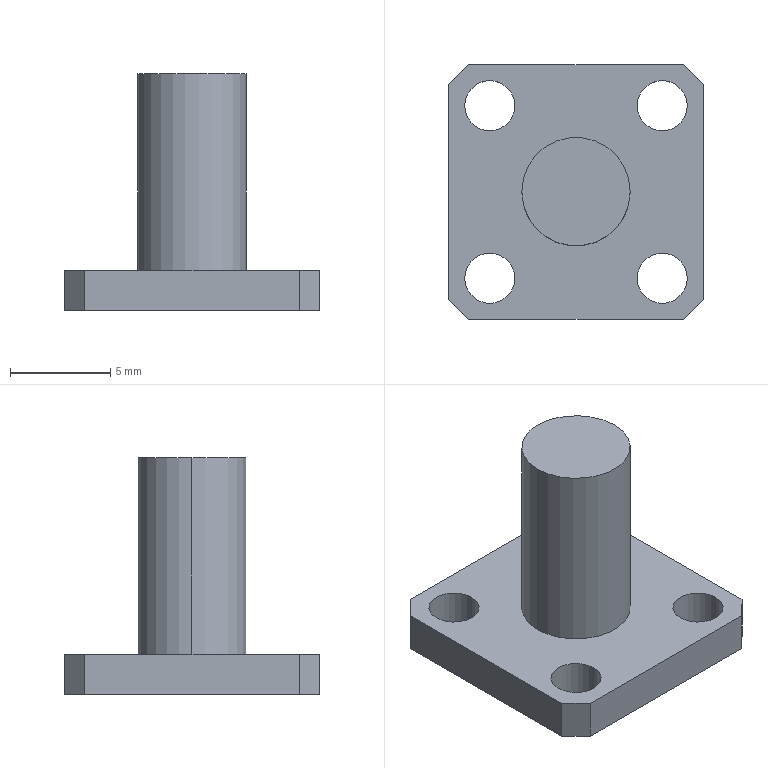Part | SolidWorks | features ICE 2, Chamfer 1, Extrusion 1 | 1 solid | 21 faces | box 12.7 x 12.7 x 11.8 mm | volume 503.752 mm3 | plane 11 | cylinder 10 | commonest cylinder face diameters 2.5 x8 5.4 x2
STEP:
#1=CARTESIAN_POINT('',(-3.65,-6.35,11.8));
#2=VERTEX_POINT('',#1);
#3=CARTESIAN_POINT('',(-9.05,-6.35,11.8));
#4=VERTEX_POINT('',#3);
#5=CARTESIAN_POINT('',(-6.35,-6.35,11.8));
#6=DIRECTION('',(0.,0.,1.));
#7=DIRECTION('',(1.,0.,0.));
#8=AXIS2_PLACEMENT_3D('',#5,#6,#7);
#9=CIRCLE('',#8,2.7);
#10=EDGE_CURVE('',#2,#4,#9,.T.);
#11=ORIENTED_EDGE('',*,*,#10,.F.);
#12=CARTESIAN_POINT('',(-3.65,-6.35,2.));
#13=VERTEX_POINT('',#12);
#14=CARTESIAN_POINT('',(-3.65,-6.35,6.6));
#15=DIRECTION('',(0.,0.,-1.));
#16=VECTOR('',#15,1000.);
#17=LINE('',#14,#16);
#18=EDGE_CURVE('',#2,#13,#17,.T.);
#19=ORIENTED_EDGE('',*,*,#18,.T.);
#20=CARTESIAN_POINT('',(-9.05,-6.35,2.));
#21=VERTEX_POINT('',#20);
#22=CARTESIAN_POINT('',(-6.35,-6.35,2.));
#23=DIRECTION('',(0.,0.,1.));
#24=DIRECTION('',(1.,0.,0.));
#25=AXIS2_PLACEMENT_3D('',#22,#23,#24);
#26=CIRCLE('',#25,2.7);
#27=EDGE_CURVE('',#13,#21,#26,.T.);
#28=ORIENTED_EDGE('',*,*,#27,.T.);
#29=CARTESIAN_POINT('',(-9.05,-6.35,6.6));
#30=DIRECTION('',(0.,0.,-1.));
#31=VECTOR('',#30,1000.);
#32=LINE('',#29,#31);
#33=EDGE_CURVE('',#4,#21,#32,.T.);
#34=ORIENTED_EDGE('',*,*,#33,.F.);
#35=EDGE_LOOP('',(#11,#19,#28,#34));
#36=FACE_OUTER_BOUND('',#35,.T.);
#37=CARTESIAN_POINT('',(-6.35,-6.35,6.6));
#38=DIRECTION('',(0.,0.,-1.));
#39=DIRECTION('',(-1.,0.,0.));
#40=AXIS2_PLACEMENT_3D('',#37,#38,#39);
#41=CYLINDRICAL_SURFACE('',#40,2.7);
#42=ADVANCED_FACE('',(#36),#41,.T.);
#43=CARTESIAN_POINT('',(-11.9,-10.65,2.));
#44=VERTEX_POINT('',#43);
#45=CARTESIAN_POINT('',(-9.4,-10.65,2.));
#46=VERTEX_POINT('',#45);
#47=CARTESIAN_POINT('',(-10.65,-10.65,2.));
#48=DIRECTION('',(0.,0.,1.));
#49=DIRECTION('',(-1.,0.,0.));
#50=AXIS2_PLACEMENT_3D('',#47,#48,#49);
#51=CIRCLE('',#50,1.25);
#52=EDGE_CURVE('',#44,#46,#51,.T.);
#53=ORIENTED_EDGE('',*,*,#52,.T.);
#54=CARTESIAN_POINT('',(-9.4,-10.65,0.));
#55=VERTEX_POINT('',#54);
#56=CARTESIAN_POINT('',(-9.4,-10.65,2.));
#57=DIRECTION('',(0.,0.,-1.));
#58=VECTOR('',#57,1000.);
#59=LINE('',#56,#58);
#60=EDGE_CURVE('',#46,#55,#59,.T.);
#61=ORIENTED_EDGE('',*,*,#60,.T.);
#62=CARTESIAN_POINT('',(-11.9,-10.65,0.));
#63=VERTEX_POINT('',#62);
#64=CARTESIAN_POINT('',(-10.65,-10.65,0.));
#65=DIRECTION('',(0.,0.,1.));
#66=DIRECTION('',(-1.,0.,0.));
#67=AXIS2_PLACEMENT_3D('',#64,#65,#66);
#68=CIRCLE('',#67,1.25);
#69=EDGE_CURVE('',#63,#55,#68,.T.);
#70=ORIENTED_EDGE('',*,*,#69,.F.);
#71=CARTESIAN_POINT('',(-11.9,-10.65,2.));
#72=DIRECTION('',(0.,0.,-1.));
#73=VECTOR('',#72,1000.);
#74=LINE('',#71,#73);
#75=EDGE_CURVE('',#44,#63,#74,.T.);
#76=ORIENTED_EDGE('',*,*,#75,.F.);
#77=EDGE_LOOP('',(#53,#61,#70,#76));
#78=FACE_OUTER_BOUND('',#77,.T.);
#79=CARTESIAN_POINT('',(-10.65,-10.65,2.));
#80=DIRECTION('',(0.,0.,-1.));
#81=DIRECTION('',(-1.,0.,0.));
#82=AXIS2_PLACEMENT_3D('',#79,#80,#81);
#83=CYLINDRICAL_SURFACE('',#82,1.25);
#84=ADVANCED_FACE('',(#78),#83,.F.);
#85=CARTESIAN_POINT('',(-3.3,-10.65,2.));
#86=VERTEX_POINT('',#85);
#87=CARTESIAN_POINT('',(-0.8,-10.65,2.));
#88=VERTEX_POINT('',#87);
#89=CARTESIAN_POINT('',(-2.05,-10.65,2.));
#90=DIRECTION('',(0.,0.,1.));
#91=DIRECTION('',(-1.,0.,0.));
#92=AXIS2_PLACEMENT_3D('',#89,#90,#91);
#93=CIRCLE('',#92,1.25);
#94=EDGE_CURVE('',#86,#88,#93,.T.);
#95=ORIENTED_EDGE('',*,*,#94,.T.);
#96=CARTESIAN_POINT('',(-0.8,-10.65,0.));
#97=VERTEX_POINT('',#96);
#98=CARTESIAN_POINT('',(-0.8,-10.65,2.));
#99=DIRECTION('',(0.,0.,-1.));
#100=VECTOR('',#99,1000.);
#101=LINE('',#98,#100);
#102=EDGE_CURVE('',#88,#97,#101,.T.);
#103=ORIENTED_EDGE('',*,*,#102,.T.);
#104=CARTESIAN_POINT('',(-3.3,-10.65,0.));
#105=VERTEX_POINT('',#104);
#106=CARTESIAN_POINT('',(-2.05,-10.65,0.));
#107=DIRECTION('',(0.,0.,1.));
#108=DIRECTION('',(-1.,0.,0.));
#109=AXIS2_PLACEMENT_3D('',#106,#107,#108);
#110=CIRCLE('',#109,1.25);
#111=EDGE_CURVE('',#105,#97,#110,.T.);
#112=ORIENTED_EDGE('',*,*,#111,.F.);
#113=CARTESIAN_POINT('',(-3.3,-10.65,2.));
#114=DIRECTION('',(0.,0.,-1.));
#115=VECTOR('',#114,1000.);
#116=LINE('',#113,#115);
#117=EDGE_CURVE('',#86,#105,#116,.T.);
#118=ORIENTED_EDGE('',*,*,#117,.F.);
#119=EDGE_LOOP('',(#95,#103,#112,#118));
#120=FACE_OUTER_BOUND('',#119,.T.);
#121=CARTESIAN_POINT('',(-2.05,-10.65,2.));
#122=DIRECTION('',(0.,0.,-1.));
#123=DIRECTION('',(-1.,0.,0.));
#124=AXIS2_PLACEMENT_3D('',#121,#122,#123);
#125=CYLINDRICAL_SURFACE('',#124,1.25);
#126=ADVANCED_FACE('',(#120),#125,.F.);
#127=CARTESIAN_POINT('',(-3.3,-2.05,2.));
#128=VERTEX_POINT('',#127);
#129=CARTESIAN_POINT('',(-0.8,-2.05,2.));
#130=VERTEX_POINT('',#129);
#131=CARTESIAN_POINT('',(-2.05,-2.05,2.));
#132=DIRECTION('',(0.,0.,1.));
#133=DIRECTION('',(1.,0.,0.));
#134=AXIS2_PLACEMENT_3D('',#131,#132,#133);
#135=CIRCLE('',#134,1.25);
#136=EDGE_CURVE('',#128,#130,#135,.T.);
#137=ORIENTED_EDGE('',*,*,#136,.T.);
#138=CARTESIAN_POINT('',(-0.8,-2.05,0.));
#139=VERTEX_POINT('',#138);
#140=CARTESIAN_POINT('',(-0.8,-2.05,2.));
#141=DIRECTION('',(0.,0.,-1.));
#142=VECTOR('',#141,1000.);
#143=LINE('',#140,#142);
#144=EDGE_CURVE('',#130,#139,#143,.T.);
#145=ORIENTED_EDGE('',*,*,#144,.T.);
#146=CARTESIAN_POINT('',(-3.3,-2.05,0.));
#147=VERTEX_POINT('',#146);
#148=CARTESIAN_POINT('',(-2.05,-2.05,0.));
#149=DIRECTION('',(0.,0.,1.));
#150=DIRECTION('',(1.,0.,0.));
#151=AXIS2_PLACEMENT_3D('',#148,#149,#150);
#152=CIRCLE('',#151,1.25);
#153=EDGE_CURVE('',#147,#139,#152,.T.);
#154=ORIENTED_EDGE('',*,*,#153,.F.);
#155=CARTESIAN_POINT('',(-3.3,-2.05,2.));
#156=DIRECTION('',(0.,0.,-1.));
#157=VECTOR('',#156,1000.);
#158=LINE('',#155,#157);
#159=EDGE_CURVE('',#128,#147,#158,.T.);
#160=ORIENTED_EDGE('',*,*,#159,.F.);
#161=EDGE_LOOP('',(#137,#145,#154,#160));
#162=FACE_OUTER_BOUND('',#161,.T.);
#163=CARTESIAN_POINT('',(-2.05,-2.05,2.));
#164=DIRECTION('',(0.,0.,-1.));
#165=DIRECTION('',(-1.,0.,0.));
#166=AXIS2_PLACEMENT_3D('',#163,#164,#165);
#167=CYLINDRICAL_SURFACE('',#166,1.25);
#168=ADVANCED_FACE('',(#162),#167,.F.);
#169=CARTESIAN_POINT('',(-11.9,-2.05,2.));
#170=VERTEX_POINT('',#169);
#171=CARTESIAN_POINT('',(-9.4,-2.05,2.));
#172=VERTEX_POINT('',#171);
#173=CARTESIAN_POINT('',(-10.65,-2.05,2.));
#174=DIRECTION('',(0.,0.,1.));
#175=DIRECTION('',(1.,0.,0.));
#176=AXIS2_PLACEMENT_3D('',#173,#174,#175);
#177=CIRCLE('',#176,1.25);
#178=EDGE_CURVE('',#170,#172,#177,.T.);
#179=ORIENTED_EDGE('',*,*,#178,.T.);
#180=CARTESIAN_POINT('',(-9.4,-2.05,0.));
#181=VERTEX_POINT('',#180);
#182=CARTESIAN_POINT('',(-9.4,-2.05,2.));
#183=DIRECTION('',(0.,0.,-1.));
#184=VECTOR('',#183,1000.);
#185=LINE('',#182,#184);
#186=EDGE_CURVE('',#172,#181,#185,.T.);
#187=ORIENTED_EDGE('',*,*,#186,.T.);
#188=CARTESIAN_POINT('',(-11.9,-2.05,0.));
#189=VERTEX_POINT('',#188);
#190=CARTESIAN_POINT('',(-10.65,-2.05,0.));
#191=DIRECTION('',(0.,0.,1.));
#192=DIRECTION('',(1.,0.,0.));
#193=AXIS2_PLACEMENT_3D('',#190,#191,#192);
#194=CIRCLE('',#193,1.25);
#195=EDGE_CURVE('',#189,#181,#194,.T.);
#196=ORIENTED_EDGE('',*,*,#195,.F.);
#197=CARTESIAN_POINT('',(-11.9,-2.05,2.));
#198=DIRECTION('',(0.,0.,-1.));
#199=VECTOR('',#198,1000.);
#200=LINE('',#197,#199);
#201=EDGE_CURVE('',#170,#189,#200,.T.);
#202=ORIENTED_EDGE('',*,*,#201,.F.);
#203=EDGE_LOOP('',(#179,#187,#196,#202));
#204=FACE_OUTER_BOUND('',#203,.T.);
#205=CARTESIAN_POINT('',(-10.65,-2.05,2.));
#206=DIRECTION('',(0.,0.,-1.));
#207=DIRECTION('',(-1.,0.,0.));
#208=AXIS2_PLACEMENT_3D('',#205,#206,#207);
#209=CYLINDRICAL_SURFACE('',#208,1.25);
#210=ADVANCED_FACE('',(#204),#209,.F.);
#211=CARTESIAN_POINT('',(-6.35,-6.35,2.));
#212=DIRECTION('',(0.,0.,1.));
#213=DIRECTION('',(1.,0.,0.));
#214=AXIS2_PLACEMENT_3D('',#211,#212,#213);
#215=CIRCLE('',#214,2.7);
#216=EDGE_CURVE('',#21,#13,#215,.T.);
#217=ORIENTED_EDGE('',*,*,#216,.F.);
#218=ORIENTED_EDGE('',*,*,#27,.F.);
#219=EDGE_LOOP('',(#217,#218));
#220=FACE_BOUND('',#219,.T.);
#221=CARTESIAN_POINT('',(-12.7,-1.,2.));
#222=VERTEX_POINT('',#221);
#223=CARTESIAN_POINT('',(-12.7,-11.7,2.));
#224=VERTEX_POINT('',#223);
#225=CARTESIAN_POINT('',(-12.7,0.,2.));
#226=DIRECTION('',(0.,-1.,0.));
#227=VECTOR('',#226,1000.);
#228=LINE('',#225,#227);
#229=EDGE_CURVE('',#222,#224,#228,.T.);
#230=ORIENTED_EDGE('',*,*,#229,.T.);
#231=CARTESIAN_POINT('',(-11.7,-12.7,2.));
#232=VERTEX_POINT('',#231);
#233=CARTESIAN_POINT('',(-11.7,-12.7,2.));
#234=DIRECTION('',(0.7071,-0.7071,0.));
#235=VECTOR('',#234,1000.);
#236=LINE('',#233,#235);
#237=EDGE_CURVE('',#224,#232,#236,.T.);
#238=ORIENTED_EDGE('',*,*,#237,.T.);
#239=CARTESIAN_POINT('',(-1.,-12.7,2.));
#240=VERTEX_POINT('',#239);
#241=CARTESIAN_POINT('',(0.,-12.7,2.));
#242=DIRECTION('',(1.,0.,0.));
#243=VECTOR('',#242,1000.);
#244=LINE('',#241,#243);
#245=EDGE_CURVE('',#232,#240,#244,.T.);
#246=ORIENTED_EDGE('',*,*,#245,.T.);
#247=CARTESIAN_POINT('',(0.,-11.7,2.));
#248=VERTEX_POINT('',#247);
#249=CARTESIAN_POINT('',(0.,-11.7,2.));
#250=DIRECTION('',(0.7071,0.7071,0.));
#251=VECTOR('',#250,1000.);
#252=LINE('',#249,#251);
#253=EDGE_CURVE('',#240,#248,#252,.T.);
#254=ORIENTED_EDGE('',*,*,#253,.T.);
#255=CARTESIAN_POINT('',(0.,-1.,2.));
#256=VERTEX_POINT('',#255);
#257=CARTESIAN_POINT('',(0.,0.,2.));
#258=DIRECTION('',(0.,1.,0.));
#259=VECTOR('',#258,1000.);
#260=LINE('',#257,#259);
#261=EDGE_CURVE('',#248,#256,#260,.T.);
#262=ORIENTED_EDGE('',*,*,#261,.T.);
#263=CARTESIAN_POINT('',(-1.,0.,2.));
#264=VERTEX_POINT('',#263);
#265=CARTESIAN_POINT('',(-1.,0.,2.));
#266=DIRECTION('',(-0.7071,0.7071,0.));
#267=VECTOR('',#266,1000.);
#268=LINE('',#265,#267);
#269=EDGE_CURVE('',#256,#264,#268,.T.);
#270=ORIENTED_EDGE('',*,*,#269,.T.);
#271=CARTESIAN_POINT('',(-11.7,0.,2.));
#272=VERTEX_POINT('',#271);
#273=CARTESIAN_POINT('',(0.,0.,2.));
#274=DIRECTION('',(-1.,0.,0.));
#275=VECTOR('',#274,1000.);
#276=LINE('',#273,#275);
#277=EDGE_CURVE('',#264,#272,#276,.T.);
#278=ORIENTED_EDGE('',*,*,#277,.T.);
#279=CARTESIAN_POINT('',(-12.7,-1.,2.));
#280=DIRECTION('',(-0.7071,-0.7071,0.));
#281=VECTOR('',#280,1000.);
#282=LINE('',#279,#281);
#283=EDGE_CURVE('',#272,#222,#282,.T.);
#284=ORIENTED_EDGE('',*,*,#283,.T.);
#285=EDGE_LOOP('',(#230,#238,#246,#254,#262,#270,#278,#284));
#286=FACE_OUTER_BOUND('',#285,.T.);
#287=ORIENTED_EDGE('',*,*,#178,.F.);
#288=CARTESIAN_POINT('',(-10.65,-2.05,2.));
#289=DIRECTION('',(0.,0.,1.));
#290=DIRECTION('',(1.,0.,0.));
#291=AXIS2_PLACEMENT_3D('',#288,#289,#290);
#292=CIRCLE('',#291,1.25);
#293=EDGE_CURVE('',#172,#170,#292,.T.);
#294=ORIENTED_EDGE('',*,*,#293,.F.);
#295=EDGE_LOOP('',(#287,#294));
#296=FACE_BOUND('',#295,.T.);
#297=ORIENTED_EDGE('',*,*,#136,.F.);
#298=CARTESIAN_POINT('',(-2.05,-2.05,2.));
#299=DIRECTION('',(0.,0.,1.));
#300=DIRECTION('',(1.,0.,0.));
#301=AXIS2_PLACEMENT_3D('',#298,#299,#300);
#302=CIRCLE('',#301,1.25);
#303=EDGE_CURVE('',#130,#128,#302,.T.);
#304=ORIENTED_EDGE('',*,*,#303,.F.);
#305=EDGE_LOOP('',(#297,#304));
#306=FACE_BOUND('',#305,.T.);
#307=ORIENTED_EDGE('',*,*,#94,.F.);
#308=CARTESIAN_POINT('',(-2.05,-10.65,2.));
#309=DIRECTION('',(0.,0.,1.));
#310=DIRECTION('',(-1.,0.,0.));
#311=AXIS2_PLACEMENT_3D('',#308,#309,#310);
#312=CIRCLE('',#311,1.25);
#313=EDGE_CURVE('',#88,#86,#312,.T.);
#314=ORIENTED_EDGE('',*,*,#313,.F.);
#315=EDGE_LOOP('',(#307,#314));
#316=FACE_BOUND('',#315,.T.);
#317=ORIENTED_EDGE('',*,*,#52,.F.);
#318=CARTESIAN_POINT('',(-10.65,-10.65,2.));
#319=DIRECTION('',(0.,0.,1.));
#320=DIRECTION('',(-1.,0.,0.));
#321=AXIS2_PLACEMENT_3D('',#318,#319,#320);
#322=CIRCLE('',#321,1.25);
#323=EDGE_CURVE('',#46,#44,#322,.T.);
#324=ORIENTED_EDGE('',*,*,#323,.F.);
#325=EDGE_LOOP('',(#317,#324));
#326=FACE_BOUND('',#325,.T.);
#327=CARTESIAN_POINT('',(0.,0.,2.));
#328=DIRECTION('',(0.,0.,-1.));
#329=DIRECTION('',(-1.,0.,0.));
#330=AXIS2_PLACEMENT_3D('',#327,#328,#329);
#331=PLANE('',#330);
#332=ADVANCED_FACE('',(#220,#286,#296,#306,#316,#326),#331,.F.);
#333=ORIENTED_EDGE('',*,*,#111,.T.);
#334=CARTESIAN_POINT('',(-2.05,-10.65,0.));
#335=DIRECTION('',(0.,0.,1.));
#336=DIRECTION('',(-1.,0.,0.));
#337=AXIS2_PLACEMENT_3D('',#334,#335,#336);
#338=CIRCLE('',#337,1.25);
#339=EDGE_CURVE('',#97,#105,#338,.T.);
#340=ORIENTED_EDGE('',*,*,#339,.T.);
#341=EDGE_LOOP('',(#333,#340));
#342=FACE_BOUND('',#341,.T.);
#343=ORIENTED_EDGE('',*,*,#195,.T.);
#344=CARTESIAN_POINT('',(-10.65,-2.05,0.));
#345=DIRECTION('',(0.,0.,1.));
#346=DIRECTION('',(1.,0.,0.));
#347=AXIS2_PLACEMENT_3D('',#344,#345,#346);
#348=CIRCLE('',#347,1.25);
#349=EDGE_CURVE('',#181,#189,#348,.T.);
#350=ORIENTED_EDGE('',*,*,#349,.T.);
#351=EDGE_LOOP('',(#343,#350));
#352=FACE_BOUND('',#351,.T.);
#353=CARTESIAN_POINT('',(-11.7,-12.7,0.));
#354=VERTEX_POINT('',#353);
#355=CARTESIAN_POINT('',(-1.,-12.7,0.));
#356=VERTEX_POINT('',#355);
#357=CARTESIAN_POINT('',(0.,-12.7,0.));
#358=DIRECTION('',(1.,0.,0.));
#359=VECTOR('',#358,1000.);
#360=LINE('',#357,#359);
#361=EDGE_CURVE('',#354,#356,#360,.T.);
#362=ORIENTED_EDGE('',*,*,#361,.F.);
#363=CARTESIAN_POINT('',(-12.7,-11.7,0.));
#364=VERTEX_POINT('',#363);
#365=CARTESIAN_POINT('',(-12.2,-12.2,0.));
#366=DIRECTION('',(-0.7071,0.7071,0.));
#367=VECTOR('',#366,1000.);
#368=LINE('',#365,#367);
#369=EDGE_CURVE('',#354,#364,#368,.T.);
#370=ORIENTED_EDGE('',*,*,#369,.T.);
#371=CARTESIAN_POINT('',(-12.7,-1.,0.));
#372=VERTEX_POINT('',#371);
#373=CARTESIAN_POINT('',(-12.7,0.,0.));
#374=DIRECTION('',(0.,-1.,0.));
#375=VECTOR('',#374,1000.);
#376=LINE('',#373,#375);
#377=EDGE_CURVE('',#372,#364,#376,.T.);
#378=ORIENTED_EDGE('',*,*,#377,.F.);
#379=CARTESIAN_POINT('',(-11.7,0.,0.));
#380=VERTEX_POINT('',#379);
#381=CARTESIAN_POINT('',(-5.85,5.85,0.));
#382=DIRECTION('',(0.7071,0.7071,0.));
#383=VECTOR('',#382,1000.);
#384=LINE('',#381,#383);
#385=EDGE_CURVE('',#372,#380,#384,.T.);
#386=ORIENTED_EDGE('',*,*,#385,.T.);
#387=CARTESIAN_POINT('',(-1.,0.,0.));
#388=VERTEX_POINT('',#387);
#389=CARTESIAN_POINT('',(0.,0.,0.));
#390=DIRECTION('',(-1.,0.,0.));
#391=VECTOR('',#390,1000.);
#392=LINE('',#389,#391);
#393=EDGE_CURVE('',#388,#380,#392,.T.);
#394=ORIENTED_EDGE('',*,*,#393,.F.);
#395=CARTESIAN_POINT('',(0.,-1.,0.));
#396=VERTEX_POINT('',#395);
#397=CARTESIAN_POINT('',(-0.5,-0.5,0.));
#398=DIRECTION('',(0.7071,-0.7071,0.));
#399=VECTOR('',#398,1000.);
#400=LINE('',#397,#399);
#401=EDGE_CURVE('',#388,#396,#400,.T.);
#402=ORIENTED_EDGE('',*,*,#401,.T.);
#403=CARTESIAN_POINT('',(0.,-11.7,0.));
#404=VERTEX_POINT('',#403);
#405=CARTESIAN_POINT('',(0.,0.,0.));
#406=DIRECTION('',(0.,1.,0.));
#407=VECTOR('',#406,1000.);
#408=LINE('',#405,#407);
#409=EDGE_CURVE('',#404,#396,#408,.T.);
#410=ORIENTED_EDGE('',*,*,#409,.F.);
#411=CARTESIAN_POINT('',(5.85,-5.85,0.));
#412=DIRECTION('',(-0.7071,-0.7071,0.));
#413=VECTOR('',#412,1000.);
#414=LINE('',#411,#413);
#415=EDGE_CURVE('',#404,#356,#414,.T.);
#416=ORIENTED_EDGE('',*,*,#415,.T.);
#417=EDGE_LOOP('',(#362,#370,#378,#386,#394,#402,#410,#416));
#418=FACE_OUTER_BOUND('',#417,.T.);
#419=ORIENTED_EDGE('',*,*,#153,.T.);
#420=CARTESIAN_POINT('',(-2.05,-2.05,0.));
#421=DIRECTION('',(0.,0.,1.));
#422=DIRECTION('',(1.,0.,0.));
#423=AXIS2_PLACEMENT_3D('',#420,#421,#422);
#424=CIRCLE('',#423,1.25);
#425=EDGE_CURVE('',#139,#147,#424,.T.);
#426=ORIENTED_EDGE('',*,*,#425,.T.);
#427=EDGE_LOOP('',(#419,#426));
#428=FACE_BOUND('',#427,.T.);
#429=ORIENTED_EDGE('',*,*,#69,.T.);
#430=CARTESIAN_POINT('',(-10.65,-10.65,0.));
#431=DIRECTION('',(0.,0.,1.));
#432=DIRECTION('',(-1.,0.,0.));
#433=AXIS2_PLACEMENT_3D('',#430,#431,#432);
#434=CIRCLE('',#433,1.25);
#435=EDGE_CURVE('',#55,#63,#434,.T.);
#436=ORIENTED_EDGE('',*,*,#435,.T.);
#437=EDGE_LOOP('',(#429,#436));
#438=FACE_BOUND('',#437,.T.);
#439=CARTESIAN_POINT('',(0.,0.,0.));
#440=DIRECTION('',(0.,0.,-1.));
#441=DIRECTION('',(-1.,0.,0.));
#442=AXIS2_PLACEMENT_3D('',#439,#440,#441);
#443=PLANE('',#442);
#444=ADVANCED_FACE('',(#342,#352,#418,#428,#438),#443,.T.);
#445=ORIENTED_EDGE('',*,*,#261,.F.);
#446=CARTESIAN_POINT('',(0.,-11.7,2.));
#447=DIRECTION('',(0.,0.,-1.));
#448=VECTOR('',#447,1000.);
#449=LINE('',#446,#448);
#450=EDGE_CURVE('',#248,#404,#449,.T.);
#451=ORIENTED_EDGE('',*,*,#450,.T.);
#452=ORIENTED_EDGE('',*,*,#409,.T.);
#453=CARTESIAN_POINT('',(0.,-1.,2.));
#454=DIRECTION('',(0.,0.,1.));
#455=VECTOR('',#454,1000.);
#456=LINE('',#453,#455);
#457=EDGE_CURVE('',#396,#256,#456,.T.);
#458=ORIENTED_EDGE('',*,*,#457,.T.);
#459=EDGE_LOOP('',(#445,#451,#452,#458));
#460=FACE_OUTER_BOUND('',#459,.T.);
#461=CARTESIAN_POINT('',(0.,0.,2.));
#462=DIRECTION('',(-1.,0.,0.));
#463=DIRECTION('',(0.,-1.,0.));
#464=AXIS2_PLACEMENT_3D('',#461,#462,#463);
#465=PLANE('',#464);
#466=ADVANCED_FACE('',(#460),#465,.F.);
#467=ORIENTED_EDGE('',*,*,#277,.F.);
#468=CARTESIAN_POINT('',(-1.,0.,2.));
#469=DIRECTION('',(0.,0.,-1.));
#470=VECTOR('',#469,1000.);
#471=LINE('',#468,#470);
#472=EDGE_CURVE('',#264,#388,#471,.T.);
#473=ORIENTED_EDGE('',*,*,#472,.T.);
#474=ORIENTED_EDGE('',*,*,#393,.T.);
#475=CARTESIAN_POINT('',(-11.7,0.,2.));
#476=DIRECTION('',(0.,0.,1.));
#477=VECTOR('',#476,1000.);
#478=LINE('',#475,#477);
#479=EDGE_CURVE('',#380,#272,#478,.T.);
#480=ORIENTED_EDGE('',*,*,#479,.T.);
#481=EDGE_LOOP('',(#467,#473,#474,#480));
#482=FACE_OUTER_BOUND('',#481,.T.);
#483=CARTESIAN_POINT('',(0.,0.,2.));
#484=DIRECTION('',(0.,-1.,0.));
#485=DIRECTION('',(0.,0.,-1.));
#486=AXIS2_PLACEMENT_3D('',#483,#484,#485);
#487=PLANE('',#486);
#488=ADVANCED_FACE('',(#482),#487,.F.);
#489=ORIENTED_EDGE('',*,*,#377,.T.);
#490=CARTESIAN_POINT('',(-12.7,-11.7,2.));
#491=DIRECTION('',(0.,0.,1.));
#492=VECTOR('',#491,1000.);
#493=LINE('',#490,#492);
#494=EDGE_CURVE('',#364,#224,#493,.T.);
#495=ORIENTED_EDGE('',*,*,#494,.T.);
#496=ORIENTED_EDGE('',*,*,#229,.F.);
#497=CARTESIAN_POINT('',(-12.7,-1.,2.));
#498=DIRECTION('',(0.,0.,-1.));
#499=VECTOR('',#498,1000.);
#500=LINE('',#497,#499);
#501=EDGE_CURVE('',#222,#372,#500,.T.);
#502=ORIENTED_EDGE('',*,*,#501,.T.);
#503=EDGE_LOOP('',(#489,#495,#496,#502));
#504=FACE_OUTER_BOUND('',#503,.T.);
#505=CARTESIAN_POINT('',(-12.7,0.,2.));
#506=DIRECTION('',(1.,0.,0.));
#507=DIRECTION('',(0.,1.,0.));
#508=AXIS2_PLACEMENT_3D('',#505,#506,#507);
#509=PLANE('',#508);
#510=ADVANCED_FACE('',(#504),#509,.F.);
#511=ORIENTED_EDGE('',*,*,#245,.F.);
#512=CARTESIAN_POINT('',(-11.7,-12.7,2.));
#513=DIRECTION('',(0.,0.,-1.));
#514=VECTOR('',#513,1000.);
#515=LINE('',#512,#514);
#516=EDGE_CURVE('',#232,#354,#515,.T.);
#517=ORIENTED_EDGE('',*,*,#516,.T.);
#518=ORIENTED_EDGE('',*,*,#361,.T.);
#519=CARTESIAN_POINT('',(-1.,-12.7,2.));
#520=DIRECTION('',(0.,0.,1.));
#521=VECTOR('',#520,1000.);
#522=LINE('',#519,#521);
#523=EDGE_CURVE('',#356,#240,#522,.T.);
#524=ORIENTED_EDGE('',*,*,#523,.T.);
#525=EDGE_LOOP('',(#511,#517,#518,#524));
#526=FACE_OUTER_BOUND('',#525,.T.);
#527=CARTESIAN_POINT('',(0.,-12.7,2.));
#528=DIRECTION('',(0.,1.,0.));
#529=DIRECTION('',(-1.,0.,0.));
#530=AXIS2_PLACEMENT_3D('',#527,#528,#529);
#531=PLANE('',#530);
#532=ADVANCED_FACE('',(#526),#531,.F.);
#533=ORIENTED_EDGE('',*,*,#186,.F.);
#534=ORIENTED_EDGE('',*,*,#293,.T.);
#535=ORIENTED_EDGE('',*,*,#201,.T.);
#536=ORIENTED_EDGE('',*,*,#349,.F.);
#537=EDGE_LOOP('',(#533,#534,#535,#536));
#538=FACE_OUTER_BOUND('',#537,.T.);
#539=CARTESIAN_POINT('',(-10.65,-2.05,2.));
#540=DIRECTION('',(0.,0.,-1.));
#541=DIRECTION('',(-1.,0.,0.));
#542=AXIS2_PLACEMENT_3D('',#539,#540,#541);
#543=CYLINDRICAL_SURFACE('',#542,1.25);
#544=ADVANCED_FACE('',(#538),#543,.F.);
#545=ORIENTED_EDGE('',*,*,#144,.F.);
#546=ORIENTED_EDGE('',*,*,#303,.T.);
#547=ORIENTED_EDGE('',*,*,#159,.T.);
#548=ORIENTED_EDGE('',*,*,#425,.F.);
#549=EDGE_LOOP('',(#545,#546,#547,#548));
#550=FACE_OUTER_BOUND('',#549,.T.);
#551=CARTESIAN_POINT('',(-2.05,-2.05,2.));
#552=DIRECTION('',(0.,0.,-1.));
#553=DIRECTION('',(-1.,0.,0.));
#554=AXIS2_PLACEMENT_3D('',#551,#552,#553);
#555=CYLINDRICAL_SURFACE('',#554,1.25);
#556=ADVANCED_FACE('',(#550),#555,.F.);
#557=ORIENTED_EDGE('',*,*,#102,.F.);
#558=ORIENTED_EDGE('',*,*,#313,.T.);
#559=ORIENTED_EDGE('',*,*,#117,.T.);
#560=ORIENTED_EDGE('',*,*,#339,.F.);
#561=EDGE_LOOP('',(#557,#558,#559,#560));
#562=FACE_OUTER_BOUND('',#561,.T.);
#563=CARTESIAN_POINT('',(-2.05,-10.65,2.));
#564=DIRECTION('',(0.,0.,-1.));
#565=DIRECTION('',(-1.,0.,0.));
#566=AXIS2_PLACEMENT_3D('',#563,#564,#565);
#567=CYLINDRICAL_SURFACE('',#566,1.25);
#568=ADVANCED_FACE('',(#562),#567,.F.);
#569=ORIENTED_EDGE('',*,*,#60,.F.);
#570=ORIENTED_EDGE('',*,*,#323,.T.);
#571=ORIENTED_EDGE('',*,*,#75,.T.);
#572=ORIENTED_EDGE('',*,*,#435,.F.);
#573=EDGE_LOOP('',(#569,#570,#571,#572));
#574=FACE_OUTER_BOUND('',#573,.T.);
#575=CARTESIAN_POINT('',(-10.65,-10.65,2.));
#576=DIRECTION('',(0.,0.,-1.));
#577=DIRECTION('',(-1.,0.,0.));
#578=AXIS2_PLACEMENT_3D('',#575,#576,#577);
#579=CYLINDRICAL_SURFACE('',#578,1.25);
#580=ADVANCED_FACE('',(#574),#579,.F.);
#581=ORIENTED_EDGE('',*,*,#237,.F.);
#582=ORIENTED_EDGE('',*,*,#494,.F.);
#583=ORIENTED_EDGE('',*,*,#369,.F.);
#584=ORIENTED_EDGE('',*,*,#516,.F.);
#585=EDGE_LOOP('',(#581,#582,#583,#584));
#586=FACE_OUTER_BOUND('',#585,.T.);
#587=CARTESIAN_POINT('',(-11.7,-12.7,2.));
#588=DIRECTION('',(0.7071,0.7071,0.));
#589=DIRECTION('',(0.,0.,-1.));
#590=AXIS2_PLACEMENT_3D('',#587,#588,#589);
#591=PLANE('',#590);
#592=ADVANCED_FACE('',(#586),#591,.F.);
#593=ORIENTED_EDGE('',*,*,#253,.F.);
#594=ORIENTED_EDGE('',*,*,#523,.F.);
#595=ORIENTED_EDGE('',*,*,#415,.F.);
#596=ORIENTED_EDGE('',*,*,#450,.F.);
#597=EDGE_LOOP('',(#593,#594,#595,#596));
#598=FACE_OUTER_BOUND('',#597,.T.);
#599=CARTESIAN_POINT('',(0.,-11.7,2.));
#600=DIRECTION('',(-0.7071,0.7071,0.));
#601=DIRECTION('',(0.,0.,-1.));
#602=AXIS2_PLACEMENT_3D('',#599,#600,#601);
#603=PLANE('',#602);
#604=ADVANCED_FACE('',(#598),#603,.F.);
#605=ORIENTED_EDGE('',*,*,#269,.F.);
#606=ORIENTED_EDGE('',*,*,#457,.F.);
#607=ORIENTED_EDGE('',*,*,#401,.F.);
#608=ORIENTED_EDGE('',*,*,#472,.F.);
#609=EDGE_LOOP('',(#605,#606,#607,#608));
#610=FACE_OUTER_BOUND('',#609,.T.);
#611=CARTESIAN_POINT('',(-1.,0.,2.));
#612=DIRECTION('',(-0.7071,-0.7071,0.));
#613=DIRECTION('',(0.,0.,-1.));
#614=AXIS2_PLACEMENT_3D('',#611,#612,#613);
#615=PLANE('',#614);
#616=ADVANCED_FACE('',(#610),#615,.F.);
#617=ORIENTED_EDGE('',*,*,#283,.F.);
#618=ORIENTED_EDGE('',*,*,#479,.F.);
#619=ORIENTED_EDGE('',*,*,#385,.F.);
#620=ORIENTED_EDGE('',*,*,#501,.F.);
#621=EDGE_LOOP('',(#617,#618,#619,#620));
#622=FACE_OUTER_BOUND('',#621,.T.);
#623=CARTESIAN_POINT('',(-12.7,-1.,2.));
#624=DIRECTION('',(0.7071,-0.7071,0.));
#625=DIRECTION('',(0.,0.,-1.));
#626=AXIS2_PLACEMENT_3D('',#623,#624,#625);
#627=PLANE('',#626);
#628=ADVANCED_FACE('',(#622),#627,.F.);
#629=ORIENTED_EDGE('',*,*,#18,.F.);
#630=CARTESIAN_POINT('',(-6.35,-6.35,11.8));
#631=DIRECTION('',(0.,0.,1.));
#632=DIRECTION('',(1.,0.,0.));
#633=AXIS2_PLACEMENT_3D('',#630,#631,#632);
#634=CIRCLE('',#633,2.7);
#635=EDGE_CURVE('',#4,#2,#634,.T.);
#636=ORIENTED_EDGE('',*,*,#635,.F.);
#637=ORIENTED_EDGE('',*,*,#33,.T.);
#638=ORIENTED_EDGE('',*,*,#216,.T.);
#639=EDGE_LOOP('',(#629,#636,#637,#638));
#640=FACE_OUTER_BOUND('',#639,.T.);
#641=CARTESIAN_POINT('',(-6.35,-6.35,6.6));
#642=DIRECTION('',(0.,0.,-1.));
#643=DIRECTION('',(-1.,0.,0.));
#644=AXIS2_PLACEMENT_3D('',#641,#642,#643);
#645=CYLINDRICAL_SURFACE('',#644,2.7);
#646=ADVANCED_FACE('',(#640),#645,.T.);
#647=ORIENTED_EDGE('',*,*,#635,.T.);
#648=ORIENTED_EDGE('',*,*,#10,.T.);
#649=EDGE_LOOP('',(#647,#648));
#650=FACE_OUTER_BOUND('',#649,.T.);
#651=CARTESIAN_POINT('',(-6.35,-6.35,11.8));
#652=DIRECTION('',(0.,0.,1.));
#653=DIRECTION('',(1.,0.,0.));
#654=AXIS2_PLACEMENT_3D('',#651,#652,#653);
#655=PLANE('',#654);
#656=ADVANCED_FACE('',(#650),#655,.T.);
#657=CLOSED_SHELL('',(#42,#84,#126,#168,#210,#332,#444,#466,#488,#510,#532,#544,#556,#568,#580,#592,#604,#616,#628,#646,#656));
#658=MANIFOLD_SOLID_BREP('',#657);
#659=CARTESIAN_POINT('',(0.,0.,0.));
#660=DIRECTION('',(0.,0.,1.));
#661=DIRECTION('',(1.,0.,0.));
#662=AXIS2_PLACEMENT_3D('',#659,#660,#661);
#663=(LENGTH_UNIT()NAMED_UNIT(*)SI_UNIT(.MILLI.,.METRE.));
#664=UNCERTAINTY_MEASURE_WITH_UNIT(LENGTH_MEASURE(0.00001),#663,'','');
#665=(NAMED_UNIT(*)PLANE_ANGLE_UNIT()SI_UNIT($,.RADIAN.));
#666=(NAMED_UNIT(*)SI_UNIT($,.STERADIAN.)SOLID_ANGLE_UNIT());
#667=(GEOMETRIC_REPRESENTATION_CONTEXT(3)GLOBAL_UNCERTAINTY_ASSIGNED_CONTEXT((#664))GLOBAL_UNIT_ASSIGNED_CONTEXT((#663,#665,#666))REPRESENTATION_CONTEXT('',''));
#668=ADVANCED_BREP_SHAPE_REPRESENTATION('',(#658,#662),#667);